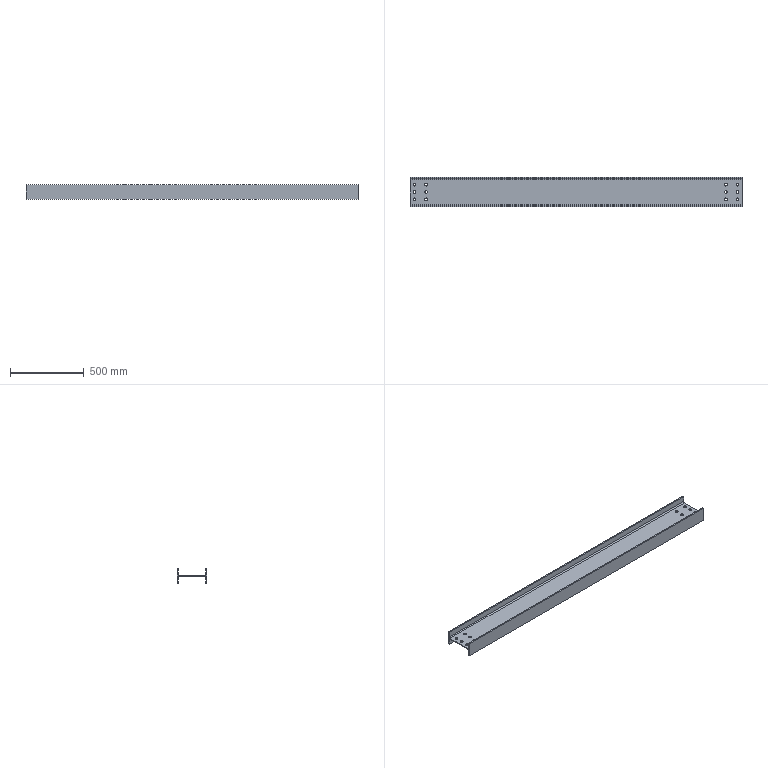Part | STEP file | 粉仓主梁13主体_Default<As Machined> | 1 solid | 42 faces | box 2255 x 200 x 100 mm | volume 5995232 mm3 | cylinder 28 | plane 14 | commonest cylinder face diameters 19 x24 16 x4